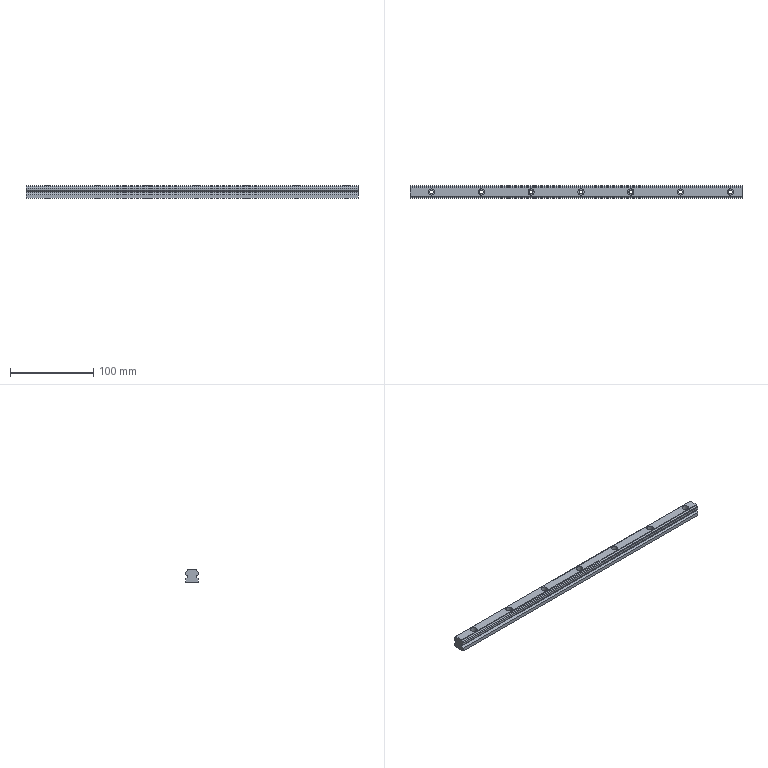Part | STEP file | Tube feed_id642_x_t | 1 solid | 43 faces | box 400 x 15 x 15 mm | volume 78237 mm3 | cylinder 22 | plane 21 | commonest cylinder face diameters 4.5 x7 7.6 x7 3 x6 1 x2